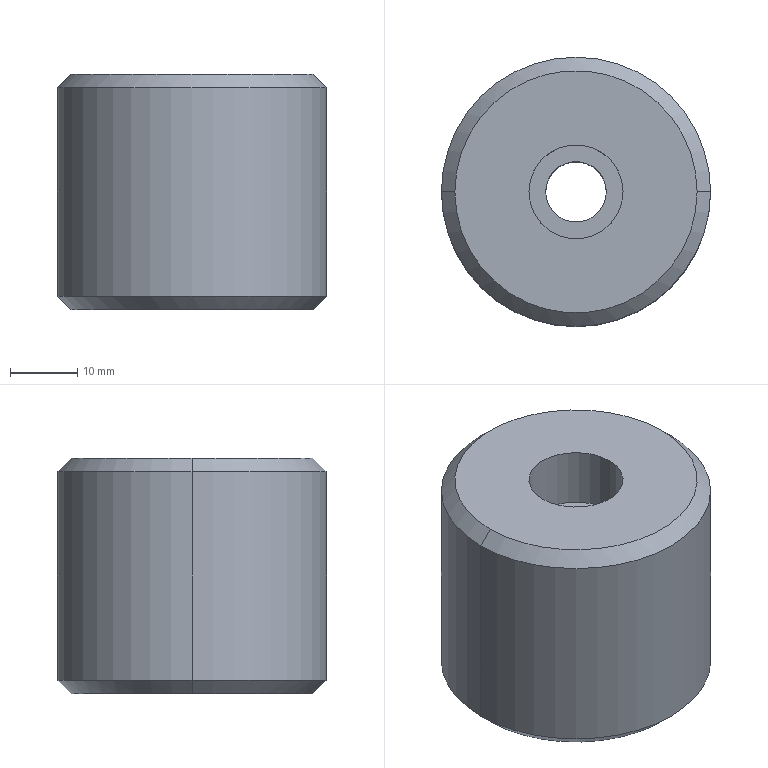Part | Creo | 1 solid | 13 faces | box 40 x 40 x 35 mm | volume 40457 mm3 | cylinder 6 | cone 4 | plane 3 | commonest cylinder face diameters 9 x2 14 x2 40 x2
STEP:
#1=CARTESIAN_POINT('',(128.,200.,-210.5));
#2=VERTEX_POINT('',#1);
#3=CARTESIAN_POINT('',(92.,200.,-210.5));
#4=VERTEX_POINT('',#3);
#5=CARTESIAN_POINT('',(110.,200.,-210.5));
#6=DIRECTION('',(0.,0.,-1.));
#7=DIRECTION('',(1.,0.,0.));
#8=AXIS2_PLACEMENT_3D('',#5,#6,#7);
#9=CIRCLE('',#8,18.);
#10=EDGE_CURVE('',#2,#4,#9,.T.);
#11=ORIENTED_EDGE('',*,*,#10,.F.);
#12=CARTESIAN_POINT('',(110.,200.,-210.5));
#13=DIRECTION('',(0.,0.,-1.));
#14=DIRECTION('',(-1.,0.,0.));
#15=AXIS2_PLACEMENT_3D('',#12,#13,#14);
#16=CIRCLE('',#15,18.);
#17=EDGE_CURVE('',#4,#2,#16,.T.);
#18=ORIENTED_EDGE('',*,*,#17,.F.);
#19=EDGE_LOOP('',(#11,#18));
#20=FACE_OUTER_BOUND('',#19,.F.);
#21=CARTESIAN_POINT('',(114.5,200.,-210.5));
#22=VERTEX_POINT('',#21);
#23=CARTESIAN_POINT('',(105.5,200.,-210.5));
#24=VERTEX_POINT('',#23);
#25=CARTESIAN_POINT('',(110.,200.,-210.5));
#26=DIRECTION('',(0.,0.,1.));
#27=DIRECTION('',(1.,0.,0.));
#28=AXIS2_PLACEMENT_3D('',#25,#26,#27);
#29=CIRCLE('',#28,4.5);
#30=EDGE_CURVE('',#22,#24,#29,.T.);
#31=ORIENTED_EDGE('',*,*,#30,.F.);
#32=CARTESIAN_POINT('',(110.,200.,-210.5));
#33=DIRECTION('',(0.,0.,1.));
#34=DIRECTION('',(-1.,0.,0.));
#35=AXIS2_PLACEMENT_3D('',#32,#33,#34);
#36=CIRCLE('',#35,4.5);
#37=EDGE_CURVE('',#24,#22,#36,.T.);
#38=ORIENTED_EDGE('',*,*,#37,.F.);
#39=EDGE_LOOP('',(#31,#38));
#40=FACE_BOUND('',#39,.F.);
#41=CARTESIAN_POINT('',(110.,200.,-210.5));
#42=DIRECTION('',(0.,0.,1.));
#43=DIRECTION('',(1.,0.,0.));
#44=AXIS2_PLACEMENT_3D('',#41,#42,#43);
#45=PLANE('',#44);
#46=ADVANCED_FACE('',(#20,#40),#45,.F.);
#47=CARTESIAN_POINT('',(105.5,200.,-184.5));
#48=VERTEX_POINT('',#47);
#49=CARTESIAN_POINT('',(114.5,200.,-184.5));
#50=VERTEX_POINT('',#49);
#51=CARTESIAN_POINT('',(110.,200.,-184.5));
#52=DIRECTION('',(0.,0.,-1.));
#53=DIRECTION('',(-1.,0.,0.));
#54=AXIS2_PLACEMENT_3D('',#51,#52,#53);
#55=CIRCLE('',#54,4.5);
#56=EDGE_CURVE('',#48,#50,#55,.T.);
#57=ORIENTED_EDGE('',*,*,#56,.T.);
#58=CARTESIAN_POINT('',(114.5,200.,-210.5));
#59=DIRECTION('',(0.,0.,1.));
#60=VECTOR('',#59,26.);
#61=LINE('',#58,#60);
#62=EDGE_CURVE('',#22,#50,#61,.T.);
#63=ORIENTED_EDGE('',*,*,#62,.F.);
#64=ORIENTED_EDGE('',*,*,#30,.T.);
#65=CARTESIAN_POINT('',(105.5,200.,-210.5));
#66=DIRECTION('',(0.,0.,1.));
#67=VECTOR('',#66,26.);
#68=LINE('',#65,#67);
#69=EDGE_CURVE('',#24,#48,#68,.T.);
#70=ORIENTED_EDGE('',*,*,#69,.T.);
#71=EDGE_LOOP('',(#57,#63,#64,#70));
#72=FACE_OUTER_BOUND('',#71,.F.);
#73=CARTESIAN_POINT('',(110.,200.,-210.5));
#74=DIRECTION('',(0.,0.,1.));
#75=DIRECTION('',(1.,0.,0.));
#76=AXIS2_PLACEMENT_3D('',#73,#74,#75);
#77=CYLINDRICAL_SURFACE('',#76,4.5);
#78=ADVANCED_FACE('',(#72),#77,.F.);
#79=CARTESIAN_POINT('',(117.,200.,-184.5));
#80=VERTEX_POINT('',#79);
#81=CARTESIAN_POINT('',(103.,200.,-184.5));
#82=VERTEX_POINT('',#81);
#83=CARTESIAN_POINT('',(110.,200.,-184.5));
#84=DIRECTION('',(0.,0.,1.));
#85=DIRECTION('',(1.,0.,0.));
#86=AXIS2_PLACEMENT_3D('',#83,#84,#85);
#87=CIRCLE('',#86,7.);
#88=EDGE_CURVE('',#80,#82,#87,.T.);
#89=ORIENTED_EDGE('',*,*,#88,.F.);
#90=CARTESIAN_POINT('',(110.,200.,-184.5));
#91=DIRECTION('',(0.,0.,1.));
#92=DIRECTION('',(-1.,0.,0.));
#93=AXIS2_PLACEMENT_3D('',#90,#91,#92);
#94=CIRCLE('',#93,7.);
#95=EDGE_CURVE('',#82,#80,#94,.T.);
#96=ORIENTED_EDGE('',*,*,#95,.F.);
#97=EDGE_LOOP('',(#89,#96));
#98=FACE_OUTER_BOUND('',#97,.F.);
#99=CARTESIAN_POINT('',(110.,200.,-184.5));
#100=DIRECTION('',(0.,0.,-1.));
#101=DIRECTION('',(1.,0.,0.));
#102=AXIS2_PLACEMENT_3D('',#99,#100,#101);
#103=CIRCLE('',#102,4.5);
#104=EDGE_CURVE('',#50,#48,#103,.T.);
#105=ORIENTED_EDGE('',*,*,#104,.F.);
#106=ORIENTED_EDGE('',*,*,#56,.F.);
#107=EDGE_LOOP('',(#105,#106));
#108=FACE_BOUND('',#107,.F.);
#109=CARTESIAN_POINT('',(110.,200.,-184.5));
#110=DIRECTION('',(0.,0.,-1.));
#111=DIRECTION('',(-1.,0.,0.));
#112=AXIS2_PLACEMENT_3D('',#109,#110,#111);
#113=PLANE('',#112);
#114=ADVANCED_FACE('',(#98,#108),#113,.F.);
#115=ORIENTED_EDGE('',*,*,#104,.T.);
#116=ORIENTED_EDGE('',*,*,#69,.F.);
#117=ORIENTED_EDGE('',*,*,#37,.T.);
#118=ORIENTED_EDGE('',*,*,#62,.T.);
#119=EDGE_LOOP('',(#115,#116,#117,#118));
#120=FACE_OUTER_BOUND('',#119,.F.);
#121=CARTESIAN_POINT('',(110.,200.,-210.5));
#122=DIRECTION('',(0.,0.,1.));
#123=DIRECTION('',(1.,0.,0.));
#124=AXIS2_PLACEMENT_3D('',#121,#122,#123);
#125=CYLINDRICAL_SURFACE('',#124,4.5);
#126=ADVANCED_FACE('',(#120),#125,.F.);
#127=CARTESIAN_POINT('',(103.,200.,-175.5));
#128=VERTEX_POINT('',#127);
#129=CARTESIAN_POINT('',(117.,200.,-175.5));
#130=VERTEX_POINT('',#129);
#131=CARTESIAN_POINT('',(110.,200.,-175.5));
#132=DIRECTION('',(0.,0.,-1.));
#133=DIRECTION('',(-1.,0.,0.));
#134=AXIS2_PLACEMENT_3D('',#131,#132,#133);
#135=CIRCLE('',#134,7.);
#136=EDGE_CURVE('',#128,#130,#135,.T.);
#137=ORIENTED_EDGE('',*,*,#136,.T.);
#138=CARTESIAN_POINT('',(117.,200.,-184.5));
#139=DIRECTION('',(0.,0.,1.));
#140=VECTOR('',#139,9.);
#141=LINE('',#138,#140);
#142=EDGE_CURVE('',#80,#130,#141,.T.);
#143=ORIENTED_EDGE('',*,*,#142,.F.);
#144=ORIENTED_EDGE('',*,*,#88,.T.);
#145=CARTESIAN_POINT('',(103.,200.,-184.5));
#146=DIRECTION('',(0.,0.,1.));
#147=VECTOR('',#146,9.);
#148=LINE('',#145,#147);
#149=EDGE_CURVE('',#82,#128,#148,.T.);
#150=ORIENTED_EDGE('',*,*,#149,.T.);
#151=EDGE_LOOP('',(#137,#143,#144,#150));
#152=FACE_OUTER_BOUND('',#151,.F.);
#153=CARTESIAN_POINT('',(110.,200.,-184.5));
#154=DIRECTION('',(0.,0.,1.));
#155=DIRECTION('',(1.,0.,0.));
#156=AXIS2_PLACEMENT_3D('',#153,#154,#155);
#157=CYLINDRICAL_SURFACE('',#156,7.);
#158=ADVANCED_FACE('',(#152),#157,.F.);
#159=CARTESIAN_POINT('',(128.,200.,-175.5));
#160=VERTEX_POINT('',#159);
#161=CARTESIAN_POINT('',(92.,200.,-175.5));
#162=VERTEX_POINT('',#161);
#163=CARTESIAN_POINT('',(110.,200.,-175.5));
#164=DIRECTION('',(0.,0.,1.));
#165=DIRECTION('',(1.,0.,0.));
#166=AXIS2_PLACEMENT_3D('',#163,#164,#165);
#167=CIRCLE('',#166,18.);
#168=EDGE_CURVE('',#160,#162,#167,.T.);
#169=ORIENTED_EDGE('',*,*,#168,.F.);
#170=CARTESIAN_POINT('',(110.,200.,-175.5));
#171=DIRECTION('',(0.,0.,1.));
#172=DIRECTION('',(-1.,0.,0.));
#173=AXIS2_PLACEMENT_3D('',#170,#171,#172);
#174=CIRCLE('',#173,18.);
#175=EDGE_CURVE('',#162,#160,#174,.T.);
#176=ORIENTED_EDGE('',*,*,#175,.F.);
#177=EDGE_LOOP('',(#169,#176));
#178=FACE_OUTER_BOUND('',#177,.F.);
#179=CARTESIAN_POINT('',(110.,200.,-175.5));
#180=DIRECTION('',(0.,0.,-1.));
#181=DIRECTION('',(1.,0.,0.));
#182=AXIS2_PLACEMENT_3D('',#179,#180,#181);
#183=CIRCLE('',#182,7.);
#184=EDGE_CURVE('',#130,#128,#183,.T.);
#185=ORIENTED_EDGE('',*,*,#184,.F.);
#186=ORIENTED_EDGE('',*,*,#136,.F.);
#187=EDGE_LOOP('',(#185,#186));
#188=FACE_BOUND('',#187,.F.);
#189=CARTESIAN_POINT('',(110.,200.,-175.5));
#190=DIRECTION('',(0.,0.,1.));
#191=DIRECTION('',(1.,0.,0.));
#192=AXIS2_PLACEMENT_3D('',#189,#190,#191);
#193=PLANE('',#192);
#194=ADVANCED_FACE('',(#178,#188),#193,.T.);
#195=ORIENTED_EDGE('',*,*,#184,.T.);
#196=ORIENTED_EDGE('',*,*,#149,.F.);
#197=ORIENTED_EDGE('',*,*,#95,.T.);
#198=ORIENTED_EDGE('',*,*,#142,.T.);
#199=EDGE_LOOP('',(#195,#196,#197,#198));
#200=FACE_OUTER_BOUND('',#199,.F.);
#201=CARTESIAN_POINT('',(110.,200.,-184.5));
#202=DIRECTION('',(0.,0.,1.));
#203=DIRECTION('',(1.,0.,0.));
#204=AXIS2_PLACEMENT_3D('',#201,#202,#203);
#205=CYLINDRICAL_SURFACE('',#204,7.);
#206=ADVANCED_FACE('',(#200),#205,.F.);
#207=CARTESIAN_POINT('',(130.,200.,-177.5));
#208=VERTEX_POINT('',#207);
#209=CARTESIAN_POINT('',(90.,200.,-177.5));
#210=VERTEX_POINT('',#209);
#211=CARTESIAN_POINT('',(110.,200.,-177.5));
#212=DIRECTION('',(0.,0.,1.));
#213=DIRECTION('',(1.,0.,0.));
#214=AXIS2_PLACEMENT_3D('',#211,#212,#213);
#215=CIRCLE('',#214,20.);
#216=EDGE_CURVE('',#208,#210,#215,.T.);
#217=ORIENTED_EDGE('',*,*,#216,.F.);
#218=CARTESIAN_POINT('',(128.,200.,-175.5));
#219=DIRECTION('',(0.7071,0.,-0.7071));
#220=VECTOR('',#219,2.828);
#221=LINE('',#218,#220);
#222=EDGE_CURVE('',#160,#208,#221,.T.);
#223=ORIENTED_EDGE('',*,*,#222,.F.);
#224=ORIENTED_EDGE('',*,*,#168,.T.);
#225=CARTESIAN_POINT('',(92.,200.,-175.5));
#226=DIRECTION('',(-0.7071,0.,-0.7071));
#227=VECTOR('',#226,2.828);
#228=LINE('',#225,#227);
#229=EDGE_CURVE('',#162,#210,#228,.T.);
#230=ORIENTED_EDGE('',*,*,#229,.T.);
#231=EDGE_LOOP('',(#217,#223,#224,#230));
#232=FACE_OUTER_BOUND('',#231,.F.);
#233=CARTESIAN_POINT('',(110.,200.,-176.5));
#234=DIRECTION('',(0.,0.,-1.));
#235=DIRECTION('',(-1.,0.,0.));
#236=AXIS2_PLACEMENT_3D('',#233,#234,#235);
#237=CONICAL_SURFACE('',#236,19.,45.);
#238=ADVANCED_FACE('',(#232),#237,.T.);
#239=CARTESIAN_POINT('',(90.,200.,-208.5));
#240=VERTEX_POINT('',#239);
#241=CARTESIAN_POINT('',(130.,200.,-208.5));
#242=VERTEX_POINT('',#241);
#243=CARTESIAN_POINT('',(110.,200.,-208.5));
#244=DIRECTION('',(0.,0.,-1.));
#245=DIRECTION('',(-1.,0.,0.));
#246=AXIS2_PLACEMENT_3D('',#243,#244,#245);
#247=CIRCLE('',#246,20.);
#248=EDGE_CURVE('',#240,#242,#247,.T.);
#249=ORIENTED_EDGE('',*,*,#248,.T.);
#250=CARTESIAN_POINT('',(130.,200.,-177.5));
#251=DIRECTION('',(0.,0.,-1.));
#252=VECTOR('',#251,31.);
#253=LINE('',#250,#252);
#254=EDGE_CURVE('',#208,#242,#253,.T.);
#255=ORIENTED_EDGE('',*,*,#254,.F.);
#256=ORIENTED_EDGE('',*,*,#216,.T.);
#257=CARTESIAN_POINT('',(90.,200.,-177.5));
#258=DIRECTION('',(0.,0.,-1.));
#259=VECTOR('',#258,31.);
#260=LINE('',#257,#259);
#261=EDGE_CURVE('',#210,#240,#260,.T.);
#262=ORIENTED_EDGE('',*,*,#261,.T.);
#263=EDGE_LOOP('',(#249,#255,#256,#262));
#264=FACE_OUTER_BOUND('',#263,.F.);
#265=CARTESIAN_POINT('',(110.,200.,-175.5));
#266=DIRECTION('',(0.,0.,-1.));
#267=DIRECTION('',(-1.,0.,0.));
#268=AXIS2_PLACEMENT_3D('',#265,#266,#267);
#269=CYLINDRICAL_SURFACE('',#268,20.);
#270=ADVANCED_FACE('',(#264),#269,.T.);
#271=ORIENTED_EDGE('',*,*,#17,.T.);
#272=CARTESIAN_POINT('',(128.,200.,-210.5));
#273=DIRECTION('',(0.7071,0.,0.7071));
#274=VECTOR('',#273,2.828);
#275=LINE('',#272,#274);
#276=EDGE_CURVE('',#2,#242,#275,.T.);
#277=ORIENTED_EDGE('',*,*,#276,.T.);
#278=ORIENTED_EDGE('',*,*,#248,.F.);
#279=CARTESIAN_POINT('',(92.,200.,-210.5));
#280=DIRECTION('',(-0.7071,0.,0.7071));
#281=VECTOR('',#280,2.828);
#282=LINE('',#279,#281);
#283=EDGE_CURVE('',#4,#240,#282,.T.);
#284=ORIENTED_EDGE('',*,*,#283,.F.);
#285=EDGE_LOOP('',(#271,#277,#278,#284));
#286=FACE_OUTER_BOUND('',#285,.F.);
#287=CARTESIAN_POINT('',(110.,200.,-209.5));
#288=DIRECTION('',(0.,0.,1.));
#289=DIRECTION('',(1.,0.,0.));
#290=AXIS2_PLACEMENT_3D('',#287,#288,#289);
#291=CONICAL_SURFACE('',#290,19.,45.);
#292=ADVANCED_FACE('',(#286),#291,.T.);
#293=ORIENTED_EDGE('',*,*,#10,.T.);
#294=ORIENTED_EDGE('',*,*,#283,.T.);
#295=CARTESIAN_POINT('',(110.,200.,-208.5));
#296=DIRECTION('',(0.,0.,-1.));
#297=DIRECTION('',(1.,0.,0.));
#298=AXIS2_PLACEMENT_3D('',#295,#296,#297);
#299=CIRCLE('',#298,20.);
#300=EDGE_CURVE('',#242,#240,#299,.T.);
#301=ORIENTED_EDGE('',*,*,#300,.F.);
#302=ORIENTED_EDGE('',*,*,#276,.F.);
#303=EDGE_LOOP('',(#293,#294,#301,#302));
#304=FACE_OUTER_BOUND('',#303,.F.);
#305=CARTESIAN_POINT('',(110.,200.,-209.5));
#306=DIRECTION('',(0.,0.,1.));
#307=DIRECTION('',(1.,0.,0.));
#308=AXIS2_PLACEMENT_3D('',#305,#306,#307);
#309=CONICAL_SURFACE('',#308,19.,45.);
#310=ADVANCED_FACE('',(#304),#309,.T.);
#311=ORIENTED_EDGE('',*,*,#300,.T.);
#312=ORIENTED_EDGE('',*,*,#261,.F.);
#313=CARTESIAN_POINT('',(110.,200.,-177.5));
#314=DIRECTION('',(0.,0.,1.));
#315=DIRECTION('',(-1.,0.,0.));
#316=AXIS2_PLACEMENT_3D('',#313,#314,#315);
#317=CIRCLE('',#316,20.);
#318=EDGE_CURVE('',#210,#208,#317,.T.);
#319=ORIENTED_EDGE('',*,*,#318,.T.);
#320=ORIENTED_EDGE('',*,*,#254,.T.);
#321=EDGE_LOOP('',(#311,#312,#319,#320));
#322=FACE_OUTER_BOUND('',#321,.F.);
#323=CARTESIAN_POINT('',(110.,200.,-175.5));
#324=DIRECTION('',(0.,0.,-1.));
#325=DIRECTION('',(-1.,0.,0.));
#326=AXIS2_PLACEMENT_3D('',#323,#324,#325);
#327=CYLINDRICAL_SURFACE('',#326,20.);
#328=ADVANCED_FACE('',(#322),#327,.T.);
#329=ORIENTED_EDGE('',*,*,#318,.F.);
#330=ORIENTED_EDGE('',*,*,#229,.F.);
#331=ORIENTED_EDGE('',*,*,#175,.T.);
#332=ORIENTED_EDGE('',*,*,#222,.T.);
#333=EDGE_LOOP('',(#329,#330,#331,#332));
#334=FACE_OUTER_BOUND('',#333,.F.);
#335=CARTESIAN_POINT('',(110.,200.,-176.5));
#336=DIRECTION('',(0.,0.,-1.));
#337=DIRECTION('',(-1.,0.,0.));
#338=AXIS2_PLACEMENT_3D('',#335,#336,#337);
#339=CONICAL_SURFACE('',#338,19.,45.);
#340=ADVANCED_FACE('',(#334),#339,.T.);
#341=CLOSED_SHELL('',(#46,#78,#114,#126,#158,#194,#206,#238,#270,#292,#310,#328,#340));
#342=MANIFOLD_SOLID_BREP('',#341);
#343=(LENGTH_UNIT()NAMED_UNIT(*)SI_UNIT(.MILLI.,.METRE.));
#344=UNCERTAINTY_MEASURE_WITH_UNIT(LENGTH_MEASURE(0.006652),#343,'','');
#345=(NAMED_UNIT(*)PLANE_ANGLE_UNIT()SI_UNIT($,.RADIAN.));
#346=PLANE_ANGLE_MEASURE_WITH_UNIT(PLANE_ANGLE_MEASURE(0.01745),#345);
#347=(CONVERSION_BASED_UNIT('DEGREE',#346)NAMED_UNIT(*)PLANE_ANGLE_UNIT());
#348=(NAMED_UNIT(*)SI_UNIT($,.STERADIAN.)SOLID_ANGLE_UNIT());
#349=(GEOMETRIC_REPRESENTATION_CONTEXT(3)GLOBAL_UNCERTAINTY_ASSIGNED_CONTEXT((#344))GLOBAL_UNIT_ASSIGNED_CONTEXT((#343,#347,#348))REPRESENTATION_CONTEXT('',''));
#350=ADVANCED_BREP_SHAPE_REPRESENTATION('',(#342),#349);